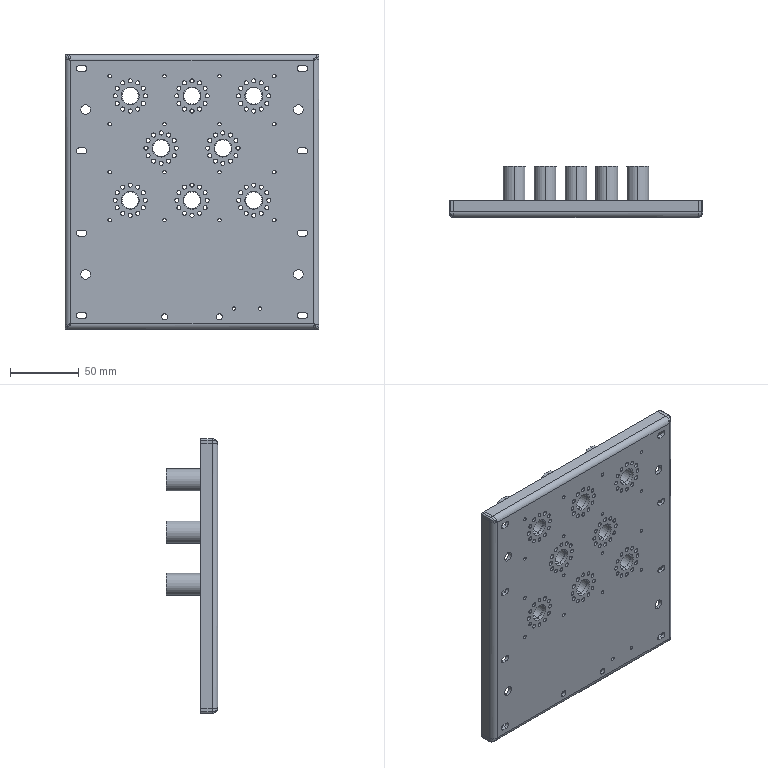Part | SolidWorks | features HoleWzd 6, SMWeldBead 4, LPattern 3, ICE 2, CirPattern 1, Cut 1, EdgeFlange 1, FlatPattern 1, MirrorPattern 1, SMBaseFlange 1, SheetMetal 1 | 1 solid | 404 faces | box 185 x 37.5 x 200 mm | volume 128218 mm3 | cylinder 318 | plane 66 | spline 20 | commonest cylinder face diameters 3 x196 2.5 x36 4.5 x20 12 x16 13 x16 16 x16